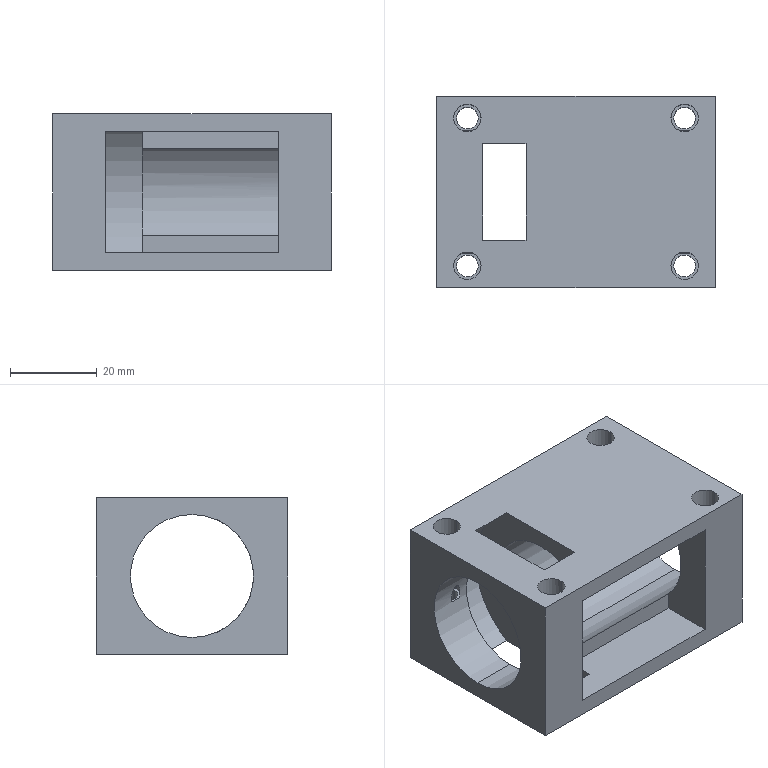Part | SolidWorks | features BaseBody 1 | 1 solid | 40 faces | box 64 x 44 x 36 mm | volume 41217 mm3 | cylinder 22 | plane 18 | commonest cylinder face diameters 5 x8 6.3 x8 28.3 x4 42.3 x2